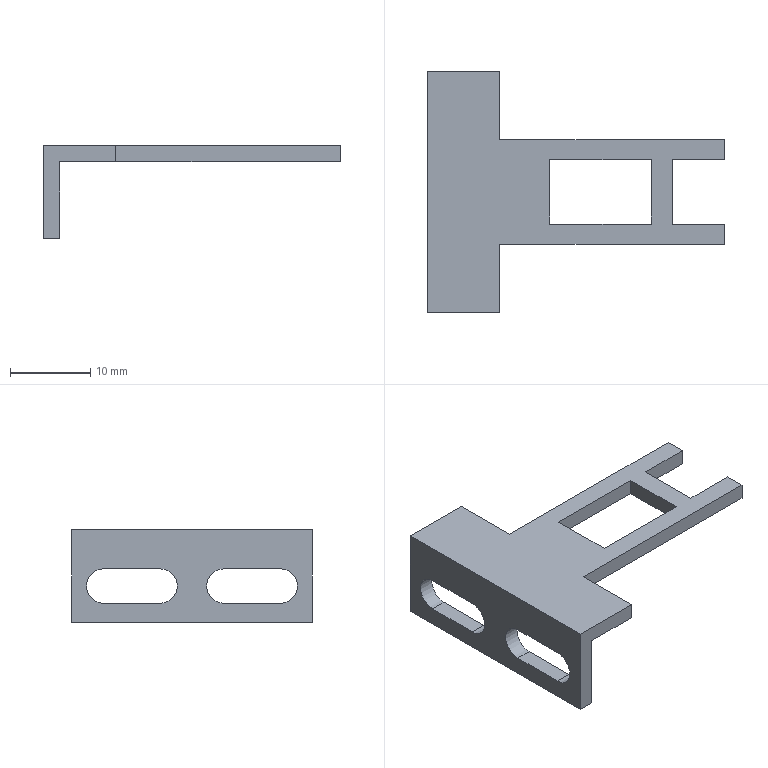Part | STEP file | D4DS_K2.step | 1 solid | 28 faces | box 37 x 30 x 11.5 mm | volume 1352 mm3 | plane 24 | cylinder 4 | commonest cylinder face diameters 4.3 x4